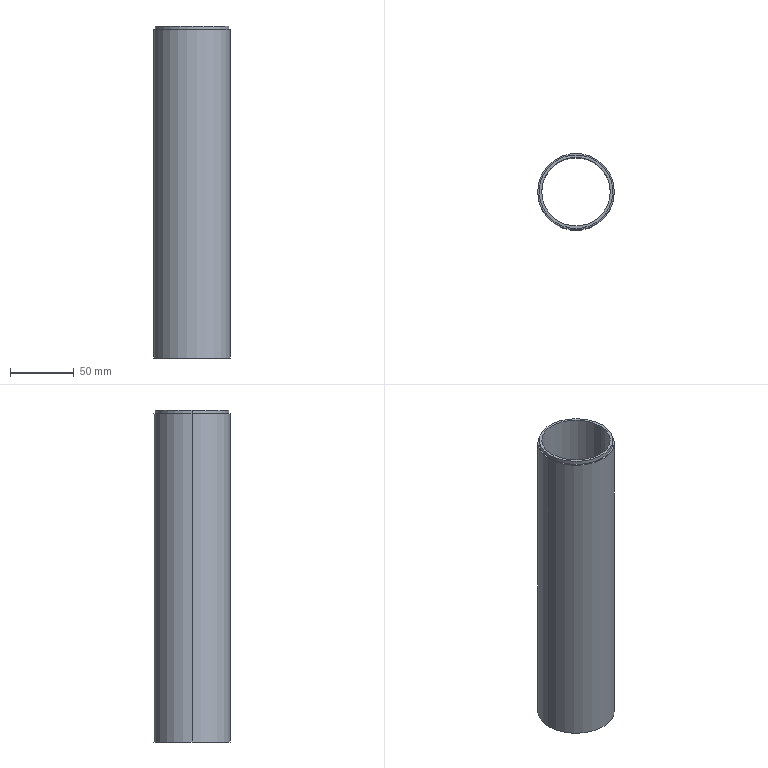Part | SolidWorks | features Extrusion 1, ICE 1, Shell 1 | 1 solid | 9 faces | box 60.3 x 60.3 x 261 mm | volume 149181 mm3 | cylinder 6 | plane 3 | commonest cylinder face diameters 53.9 x2 58 x2 60.3 x2
STEP:
#1=CARTESIAN_POINT('',(29.,0.,258.));
#2=VERTEX_POINT('',#1);
#3=CARTESIAN_POINT('',(-29.,0.,258.));
#4=VERTEX_POINT('',#3);
#5=CARTESIAN_POINT('',(0.,0.,258.));
#6=DIRECTION('',(0.,0.,1.));
#7=DIRECTION('',(1.,0.,0.));
#8=AXIS2_PLACEMENT_3D('',#5,#6,#7);
#9=CIRCLE('',#8,29.);
#10=EDGE_CURVE('',#2,#4,#9,.T.);
#11=ORIENTED_EDGE('',*,*,#10,.T.);
#12=CARTESIAN_POINT('',(-29.,0.,261.));
#13=VERTEX_POINT('',#12);
#14=CARTESIAN_POINT('',(-29.,0.,258.));
#15=DIRECTION('',(0.,0.,1.));
#16=VECTOR('',#15,1000.);
#17=LINE('',#14,#16);
#18=EDGE_CURVE('',#4,#13,#17,.T.);
#19=ORIENTED_EDGE('',*,*,#18,.T.);
#20=CARTESIAN_POINT('',(29.,0.,261.));
#21=VERTEX_POINT('',#20);
#22=CARTESIAN_POINT('',(0.,0.,261.));
#23=DIRECTION('',(0.,0.,1.));
#24=DIRECTION('',(1.,0.,0.));
#25=AXIS2_PLACEMENT_3D('',#22,#23,#24);
#26=CIRCLE('',#25,29.);
#27=EDGE_CURVE('',#21,#13,#26,.T.);
#28=ORIENTED_EDGE('',*,*,#27,.F.);
#29=CARTESIAN_POINT('',(29.,0.,258.));
#30=DIRECTION('',(0.,0.,1.));
#31=VECTOR('',#30,1000.);
#32=LINE('',#29,#31);
#33=EDGE_CURVE('',#2,#21,#32,.T.);
#34=ORIENTED_EDGE('',*,*,#33,.F.);
#35=EDGE_LOOP('',(#11,#19,#28,#34));
#36=FACE_OUTER_BOUND('',#35,.T.);
#37=CARTESIAN_POINT('',(0.,0.,258.));
#38=DIRECTION('',(0.,0.,1.));
#39=DIRECTION('',(1.,0.,0.));
#40=AXIS2_PLACEMENT_3D('',#37,#38,#39);
#41=CYLINDRICAL_SURFACE('',#40,29.);
#42=ADVANCED_FACE('',(#36),#41,.T.);
#43=CARTESIAN_POINT('',(-26.95,0.,261.));
#44=VERTEX_POINT('',#43);
#45=CARTESIAN_POINT('',(26.95,0.,261.));
#46=VERTEX_POINT('',#45);
#47=CARTESIAN_POINT('',(0.,0.,261.));
#48=DIRECTION('',(0.,0.,1.));
#49=DIRECTION('',(1.,0.,0.));
#50=AXIS2_PLACEMENT_3D('',#47,#48,#49);
#51=CIRCLE('',#50,26.95);
#52=EDGE_CURVE('',#44,#46,#51,.T.);
#53=ORIENTED_EDGE('',*,*,#52,.T.);
#54=CARTESIAN_POINT('',(26.95,0.,0.));
#55=VERTEX_POINT('',#54);
#56=CARTESIAN_POINT('',(26.95,0.,261.));
#57=DIRECTION('',(0.,0.,-1.));
#58=VECTOR('',#57,1000.);
#59=LINE('',#56,#58);
#60=EDGE_CURVE('',#46,#55,#59,.T.);
#61=ORIENTED_EDGE('',*,*,#60,.T.);
#62=CARTESIAN_POINT('',(-26.95,0.,0.));
#63=VERTEX_POINT('',#62);
#64=CARTESIAN_POINT('',(0.,0.,0.));
#65=DIRECTION('',(0.,0.,1.));
#66=DIRECTION('',(1.,0.,0.));
#67=AXIS2_PLACEMENT_3D('',#64,#65,#66);
#68=CIRCLE('',#67,26.95);
#69=EDGE_CURVE('',#63,#55,#68,.T.);
#70=ORIENTED_EDGE('',*,*,#69,.F.);
#71=CARTESIAN_POINT('',(-26.95,0.,261.));
#72=DIRECTION('',(0.,0.,-1.));
#73=VECTOR('',#72,1000.);
#74=LINE('',#71,#73);
#75=EDGE_CURVE('',#44,#63,#74,.T.);
#76=ORIENTED_EDGE('',*,*,#75,.F.);
#77=EDGE_LOOP('',(#53,#61,#70,#76));
#78=FACE_OUTER_BOUND('',#77,.T.);
#79=CARTESIAN_POINT('',(0.,0.,261.));
#80=DIRECTION('',(0.,0.,-1.));
#81=DIRECTION('',(-1.,0.,0.));
#82=AXIS2_PLACEMENT_3D('',#79,#80,#81);
#83=CYLINDRICAL_SURFACE('',#82,26.95);
#84=ADVANCED_FACE('',(#78),#83,.F.);
#85=CARTESIAN_POINT('',(30.15,0.,258.));
#86=VERTEX_POINT('',#85);
#87=CARTESIAN_POINT('',(-30.15,0.,258.));
#88=VERTEX_POINT('',#87);
#89=CARTESIAN_POINT('',(0.,0.,258.));
#90=DIRECTION('',(0.,0.,1.));
#91=DIRECTION('',(1.,0.,0.));
#92=AXIS2_PLACEMENT_3D('',#89,#90,#91);
#93=CIRCLE('',#92,30.15);
#94=EDGE_CURVE('',#86,#88,#93,.T.);
#95=ORIENTED_EDGE('',*,*,#94,.F.);
#96=CARTESIAN_POINT('',(30.15,0.,0.));
#97=VERTEX_POINT('',#96);
#98=CARTESIAN_POINT('',(30.15,0.,261.));
#99=DIRECTION('',(0.,0.,-1.));
#100=VECTOR('',#99,1000.);
#101=LINE('',#98,#100);
#102=EDGE_CURVE('',#86,#97,#101,.T.);
#103=ORIENTED_EDGE('',*,*,#102,.T.);
#104=CARTESIAN_POINT('',(-30.15,0.,0.));
#105=VERTEX_POINT('',#104);
#106=CARTESIAN_POINT('',(0.,0.,0.));
#107=DIRECTION('',(0.,0.,1.));
#108=DIRECTION('',(1.,0.,0.));
#109=AXIS2_PLACEMENT_3D('',#106,#107,#108);
#110=CIRCLE('',#109,30.15);
#111=EDGE_CURVE('',#97,#105,#110,.T.);
#112=ORIENTED_EDGE('',*,*,#111,.T.);
#113=CARTESIAN_POINT('',(-30.15,0.,261.));
#114=DIRECTION('',(0.,0.,-1.));
#115=VECTOR('',#114,1000.);
#116=LINE('',#113,#115);
#117=EDGE_CURVE('',#88,#105,#116,.T.);
#118=ORIENTED_EDGE('',*,*,#117,.F.);
#119=EDGE_LOOP('',(#95,#103,#112,#118));
#120=FACE_OUTER_BOUND('',#119,.T.);
#121=CARTESIAN_POINT('',(0.,0.,261.));
#122=DIRECTION('',(0.,0.,-1.));
#123=DIRECTION('',(-1.,0.,0.));
#124=AXIS2_PLACEMENT_3D('',#121,#122,#123);
#125=CYLINDRICAL_SURFACE('',#124,30.15);
#126=ADVANCED_FACE('',(#120),#125,.T.);
#127=ORIENTED_EDGE('',*,*,#102,.F.);
#128=CARTESIAN_POINT('',(0.,0.,258.));
#129=DIRECTION('',(0.,0.,1.));
#130=DIRECTION('',(1.,0.,0.));
#131=AXIS2_PLACEMENT_3D('',#128,#129,#130);
#132=CIRCLE('',#131,30.15);
#133=EDGE_CURVE('',#88,#86,#132,.T.);
#134=ORIENTED_EDGE('',*,*,#133,.F.);
#135=ORIENTED_EDGE('',*,*,#117,.T.);
#136=CARTESIAN_POINT('',(0.,0.,0.));
#137=DIRECTION('',(0.,0.,1.));
#138=DIRECTION('',(1.,0.,0.));
#139=AXIS2_PLACEMENT_3D('',#136,#137,#138);
#140=CIRCLE('',#139,30.15);
#141=EDGE_CURVE('',#105,#97,#140,.T.);
#142=ORIENTED_EDGE('',*,*,#141,.T.);
#143=EDGE_LOOP('',(#127,#134,#135,#142));
#144=FACE_OUTER_BOUND('',#143,.T.);
#145=CARTESIAN_POINT('',(0.,0.,261.));
#146=DIRECTION('',(0.,0.,-1.));
#147=DIRECTION('',(-1.,0.,0.));
#148=AXIS2_PLACEMENT_3D('',#145,#146,#147);
#149=CYLINDRICAL_SURFACE('',#148,30.15);
#150=ADVANCED_FACE('',(#144),#149,.T.);
#151=ORIENTED_EDGE('',*,*,#52,.F.);
#152=CARTESIAN_POINT('',(0.,0.,261.));
#153=DIRECTION('',(0.,0.,1.));
#154=DIRECTION('',(1.,0.,0.));
#155=AXIS2_PLACEMENT_3D('',#152,#153,#154);
#156=CIRCLE('',#155,26.95);
#157=EDGE_CURVE('',#46,#44,#156,.T.);
#158=ORIENTED_EDGE('',*,*,#157,.F.);
#159=EDGE_LOOP('',(#151,#158));
#160=FACE_BOUND('',#159,.T.);
#161=ORIENTED_EDGE('',*,*,#27,.T.);
#162=CARTESIAN_POINT('',(0.,0.,261.));
#163=DIRECTION('',(0.,0.,1.));
#164=DIRECTION('',(1.,0.,0.));
#165=AXIS2_PLACEMENT_3D('',#162,#163,#164);
#166=CIRCLE('',#165,29.);
#167=EDGE_CURVE('',#13,#21,#166,.T.);
#168=ORIENTED_EDGE('',*,*,#167,.T.);
#169=EDGE_LOOP('',(#161,#168));
#170=FACE_OUTER_BOUND('',#169,.T.);
#171=CARTESIAN_POINT('',(0.,0.,261.));
#172=DIRECTION('',(0.,0.,1.));
#173=DIRECTION('',(1.,0.,0.));
#174=AXIS2_PLACEMENT_3D('',#171,#172,#173);
#175=PLANE('',#174);
#176=ADVANCED_FACE('',(#160,#170),#175,.T.);
#177=ORIENTED_EDGE('',*,*,#69,.T.);
#178=CARTESIAN_POINT('',(0.,0.,0.));
#179=DIRECTION('',(0.,0.,1.));
#180=DIRECTION('',(1.,0.,0.));
#181=AXIS2_PLACEMENT_3D('',#178,#179,#180);
#182=CIRCLE('',#181,26.95);
#183=EDGE_CURVE('',#55,#63,#182,.T.);
#184=ORIENTED_EDGE('',*,*,#183,.T.);
#185=EDGE_LOOP('',(#177,#184));
#186=FACE_BOUND('',#185,.T.);
#187=ORIENTED_EDGE('',*,*,#141,.F.);
#188=ORIENTED_EDGE('',*,*,#111,.F.);
#189=EDGE_LOOP('',(#187,#188));
#190=FACE_OUTER_BOUND('',#189,.T.);
#191=CARTESIAN_POINT('',(0.,0.,0.));
#192=DIRECTION('',(0.,0.,1.));
#193=DIRECTION('',(1.,0.,0.));
#194=AXIS2_PLACEMENT_3D('',#191,#192,#193);
#195=PLANE('',#194);
#196=ADVANCED_FACE('',(#186,#190),#195,.F.);
#197=ORIENTED_EDGE('',*,*,#60,.F.);
#198=ORIENTED_EDGE('',*,*,#157,.T.);
#199=ORIENTED_EDGE('',*,*,#75,.T.);
#200=ORIENTED_EDGE('',*,*,#183,.F.);
#201=EDGE_LOOP('',(#197,#198,#199,#200));
#202=FACE_OUTER_BOUND('',#201,.T.);
#203=CARTESIAN_POINT('',(0.,0.,261.));
#204=DIRECTION('',(0.,0.,-1.));
#205=DIRECTION('',(-1.,0.,0.));
#206=AXIS2_PLACEMENT_3D('',#203,#204,#205);
#207=CYLINDRICAL_SURFACE('',#206,26.95);
#208=ADVANCED_FACE('',(#202),#207,.F.);
#209=ORIENTED_EDGE('',*,*,#10,.F.);
#210=CARTESIAN_POINT('',(0.,0.,258.));
#211=DIRECTION('',(0.,0.,1.));
#212=DIRECTION('',(1.,0.,0.));
#213=AXIS2_PLACEMENT_3D('',#210,#211,#212);
#214=CIRCLE('',#213,29.);
#215=EDGE_CURVE('',#4,#2,#214,.T.);
#216=ORIENTED_EDGE('',*,*,#215,.F.);
#217=EDGE_LOOP('',(#209,#216));
#218=FACE_BOUND('',#217,.T.);
#219=ORIENTED_EDGE('',*,*,#133,.T.);
#220=ORIENTED_EDGE('',*,*,#94,.T.);
#221=EDGE_LOOP('',(#219,#220));
#222=FACE_OUTER_BOUND('',#221,.T.);
#223=CARTESIAN_POINT('',(0.,0.,258.));
#224=DIRECTION('',(0.,0.,1.));
#225=DIRECTION('',(1.,0.,0.));
#226=AXIS2_PLACEMENT_3D('',#223,#224,#225);
#227=PLANE('',#226);
#228=ADVANCED_FACE('',(#218,#222),#227,.T.);
#229=ORIENTED_EDGE('',*,*,#18,.F.);
#230=ORIENTED_EDGE('',*,*,#215,.T.);
#231=ORIENTED_EDGE('',*,*,#33,.T.);
#232=ORIENTED_EDGE('',*,*,#167,.F.);
#233=EDGE_LOOP('',(#229,#230,#231,#232));
#234=FACE_OUTER_BOUND('',#233,.T.);
#235=CARTESIAN_POINT('',(0.,0.,258.));
#236=DIRECTION('',(0.,0.,1.));
#237=DIRECTION('',(1.,0.,0.));
#238=AXIS2_PLACEMENT_3D('',#235,#236,#237);
#239=CYLINDRICAL_SURFACE('',#238,29.);
#240=ADVANCED_FACE('',(#234),#239,.T.);
#241=CLOSED_SHELL('',(#42,#84,#126,#150,#176,#196,#208,#228,#240));
#242=MANIFOLD_SOLID_BREP('',#241);
#243=CARTESIAN_POINT('',(0.,0.,0.));
#244=DIRECTION('',(0.,0.,1.));
#245=DIRECTION('',(1.,0.,0.));
#246=AXIS2_PLACEMENT_3D('',#243,#244,#245);
#247=(LENGTH_UNIT()NAMED_UNIT(*)SI_UNIT(.MILLI.,.METRE.));
#248=UNCERTAINTY_MEASURE_WITH_UNIT(LENGTH_MEASURE(0.00001),#247,'','');
#249=(NAMED_UNIT(*)PLANE_ANGLE_UNIT()SI_UNIT($,.RADIAN.));
#250=(NAMED_UNIT(*)SI_UNIT($,.STERADIAN.)SOLID_ANGLE_UNIT());
#251=(GEOMETRIC_REPRESENTATION_CONTEXT(3)GLOBAL_UNCERTAINTY_ASSIGNED_CONTEXT((#248))GLOBAL_UNIT_ASSIGNED_CONTEXT((#247,#249,#250))REPRESENTATION_CONTEXT('',''));
#252=ADVANCED_BREP_SHAPE_REPRESENTATION('',(#242,#246),#251);